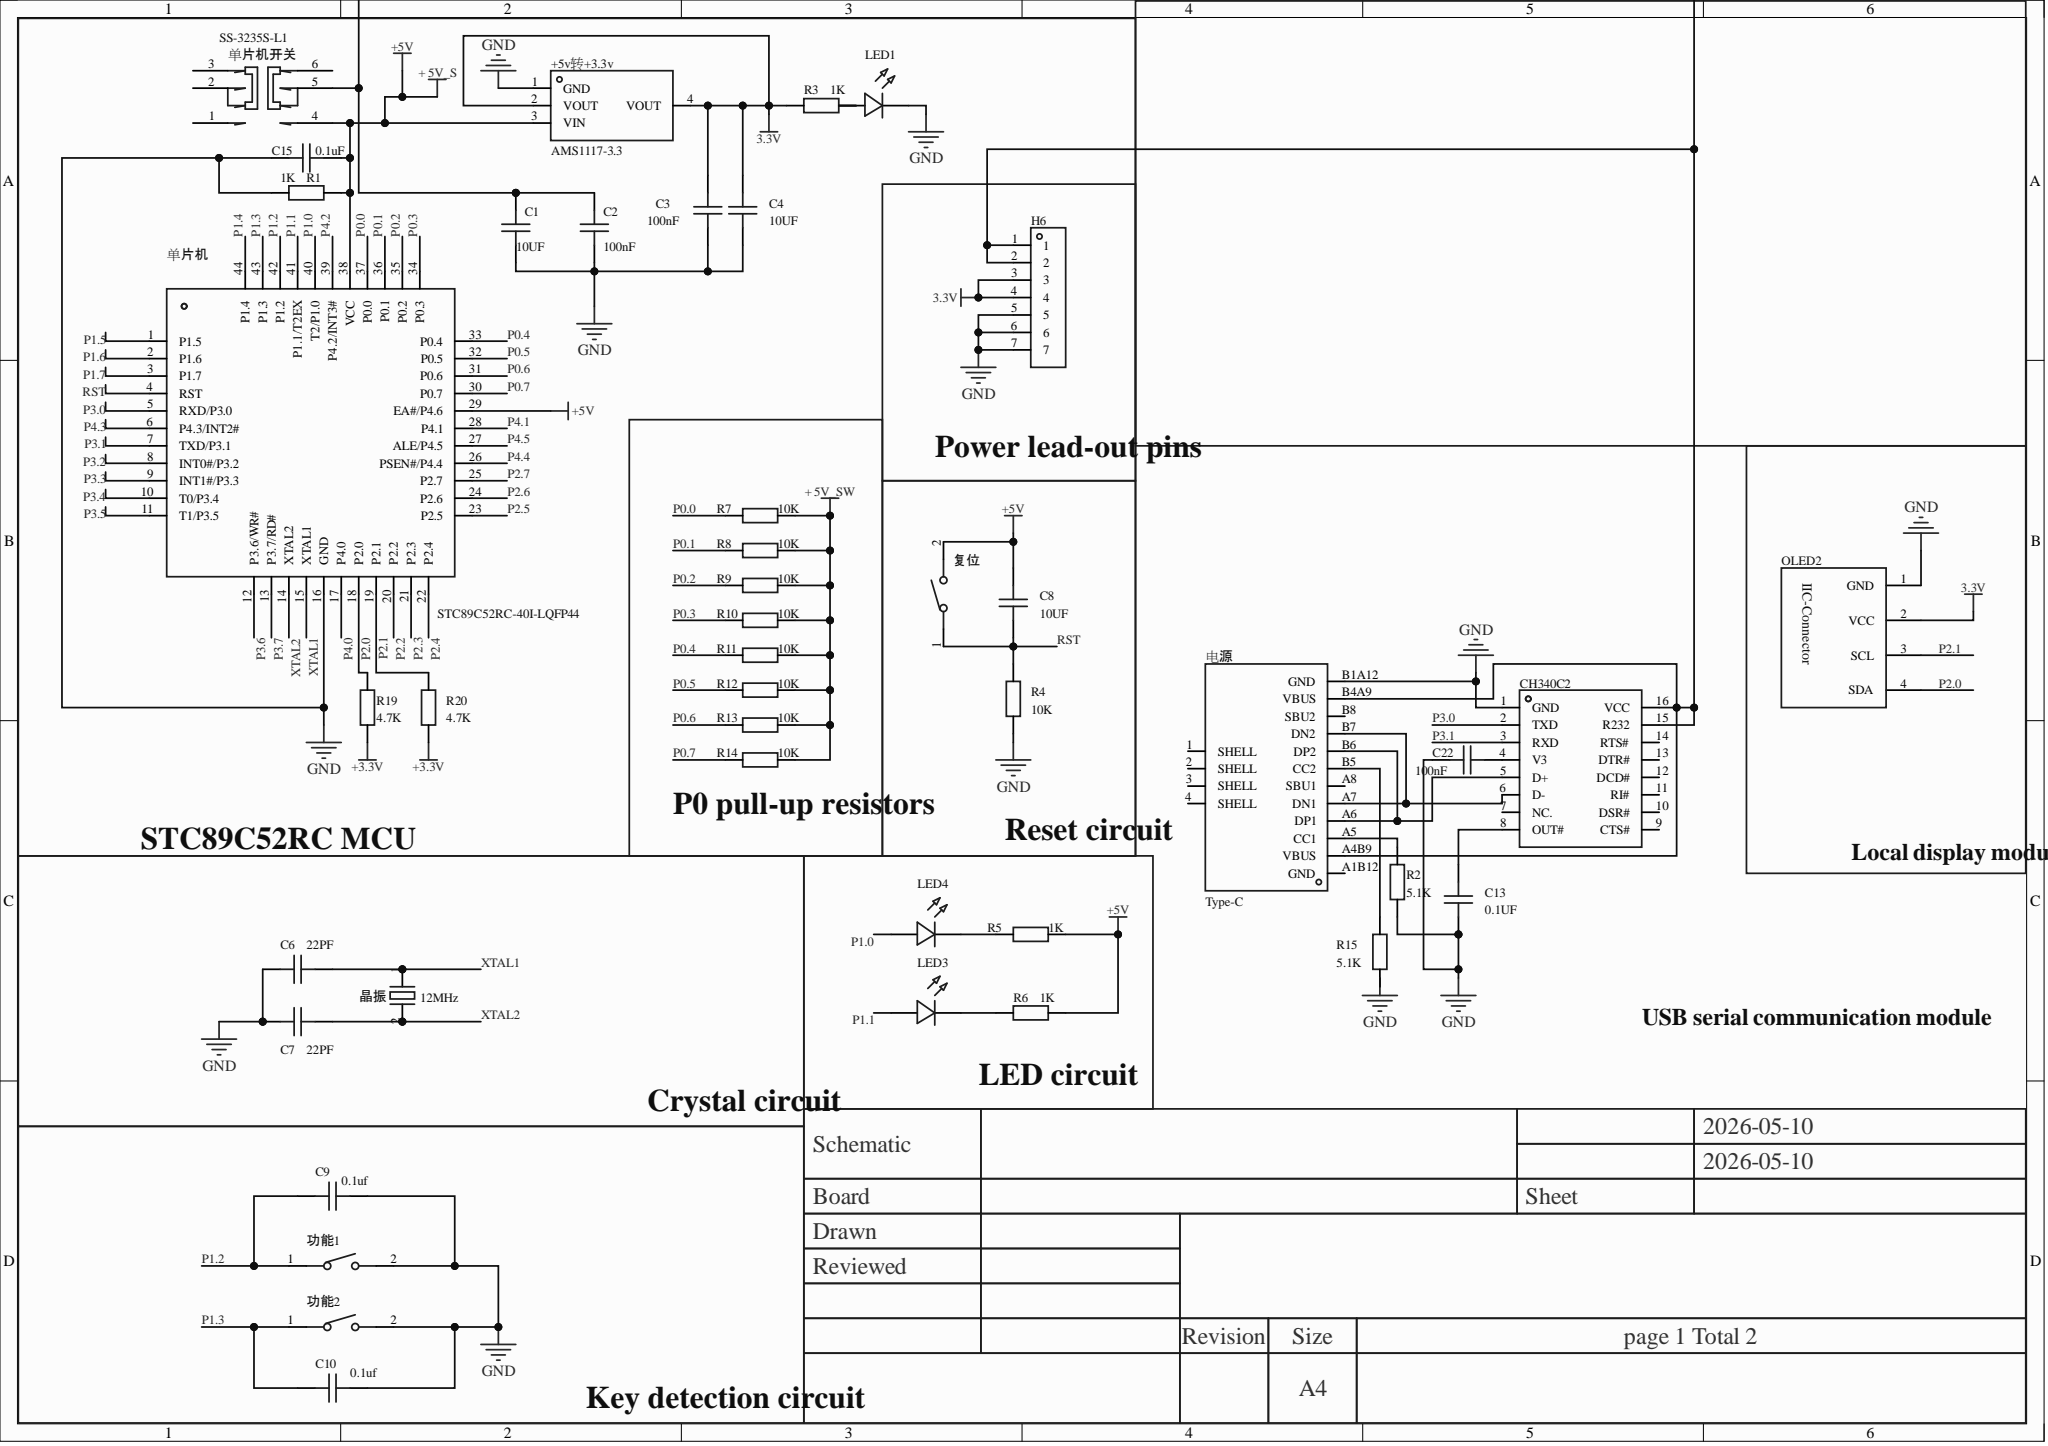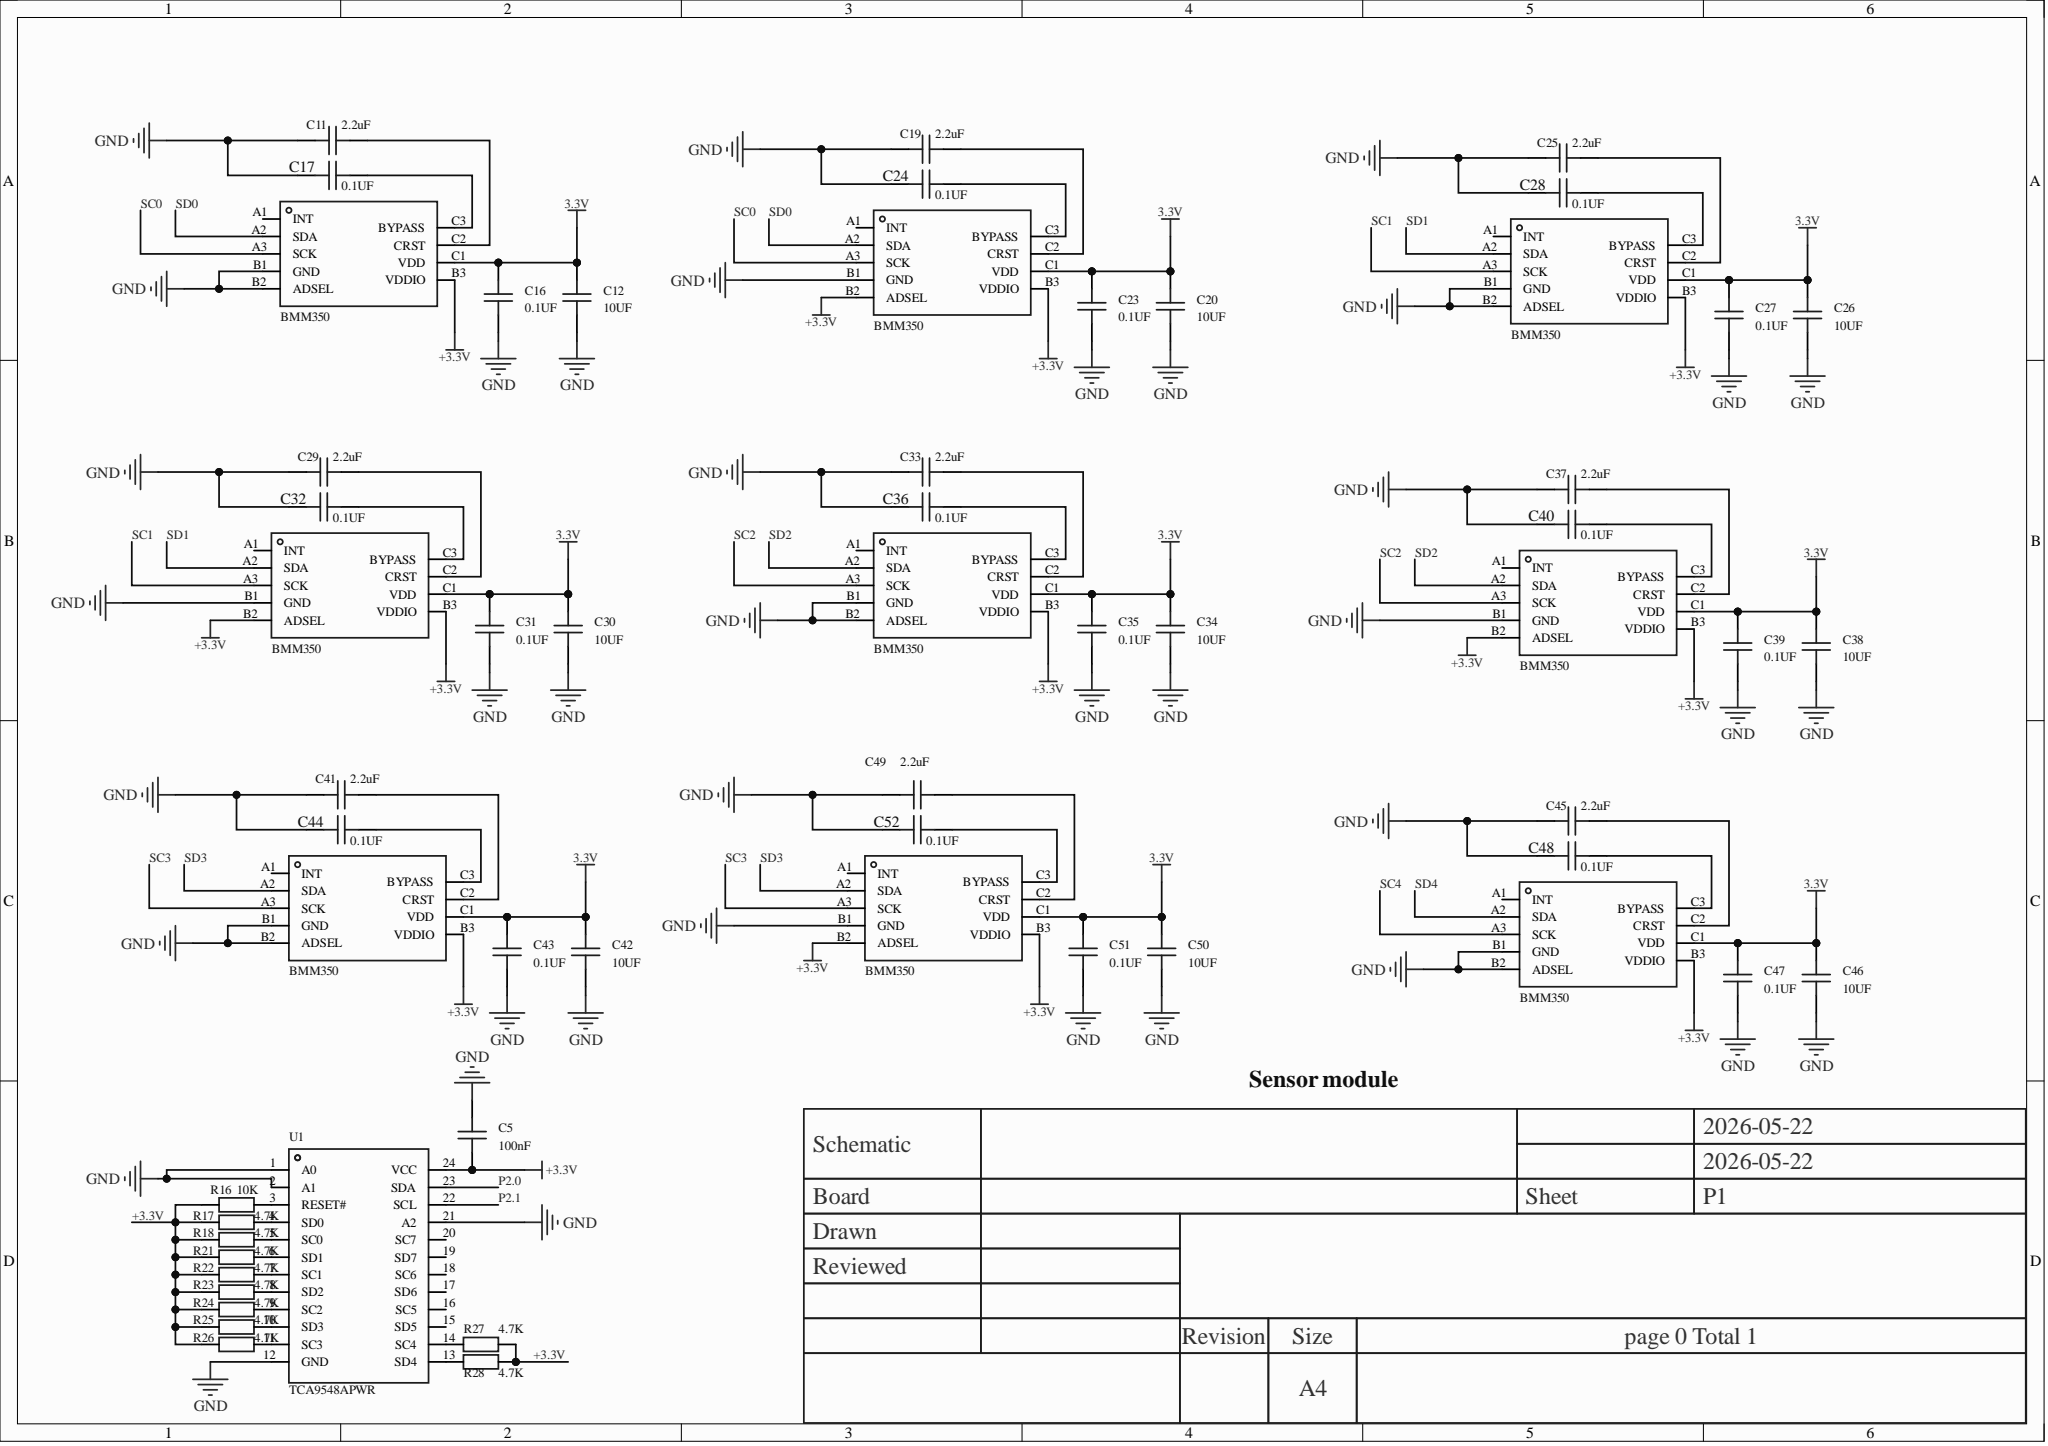Circuit board | Altium Designer | 101 parts | 69 nets
Bill of materials:
Comment,Description,Designator,Footprint,LibRef,Quantity
"AMS1117-3.3","Output type: fixed; working voltage: 15V; output voltage: 3.3V; output current: 1A; PSRR: 72dB@(120Hz); output polarity: positive;","+5v转+3.3v","SOT-223-3_L6.5-W3.4-P2.30-LS7.0-BR","AMS1117-3.3_C6186","1"
"10UF","","C1, C4, C8, C12, C20, C26, C30, C34, C38, C42, C46, C50","C0805","CAP_0805","12"
"100nF","","C2, C3, C5","C0805","CAP_0805","3"
"22PF","","C6, C7","C0805","CAP_0805","2"
"0.1uf","","C9, C10, C13, C15, C16, C17, C23, C24, C27, C28, C31, C32, C35, C36, C39, C40, C43, C44, C47, C48, C51, C52","C0805","CAP_0805","22"
"2.2uF","Capacitance: 2.2uF; tolerance: ±10%; rated voltage: 6.3V; dielectric (temperature coefficient): X7R;","C11, C19, C25, C29, C33, C37, C41, C45, C49","C0805","CGB4B3X7R0J225K055AB","9"
"100nF","","C22","C0603","CAP_0603","1"
"CH340C","Application function: transceiver; USB protocol version: USB 2.0; data rate: 2Mbps;","CH340C2","SOP-16_L10.0-W3.9-P1.27-LS6.0-BL","CH340C","1"
"","","H6","HDR-TH_7P-P2.54-V-M","HDR-M_2.54_1x7P","1"
"","","LED1, LED3, LED4","LED_0805","LED_0805-G","3"
"0.96OLED_4P_MODULE_JX","","OLED2","0.96OLED_4P","0.96OLED_4P_MODULE_JX","1"
"1K","","R1, R3, R5, R6","R0805","Res_0805","4"
"5.1K","","R2, R15","R0603","Res_0603","2"
"10K","","R4, R7, R8, R9, R10, R11, R12, R13, R14, R16","R0805","Res_0805","10"
"4.7K","","R17, R18, R21, R22, R23, R24, R25, R26, R27, R28","R0805","Res_0805","10"
"4.7K","","R19, R20","R0603","Res_0603","2"
"TCA9548APWR","TCA9548A 8-channel, 1.65V to 5.5V I2C/SMBus switch with reset and voltage translation","U1","TSSOP-24_L7.8-W4.4-P0.65-LS6.4-BL","TCA9548APWR","1"
"BMM350","","U2, U3, U4, U5, U6, U7, U8, U9, U10","WLCSP-9_L1.3-W1.3-R3-C3-P0.40-TL","BMM350","9"
"Tact switch 3*4*H","","功能1, 功能2, 复位","SW-SMD_L4.0-W2.9-LS5.0","轻触按键3*4*H","3"
"STC89C52RC-40I-LQFP44","CPU core: 51 family;","单片机","LQFP-44_L10.0-W10.0-P0.80-LS12.0-BL","STC89C52RC-40I-LQFP44","1"
"SS-3235S-L1","Circuit: DPDT; mounting: flat mount; switch colour: black; rated current: 50mA; rated voltage: 12V; service life: 1万 cycles;","单片机开关","SW-SMD_SS-3235S-LX","SS-3235S-L1","1"
"12MHz","Frequency: 12MHz; frequency tolerance at room temperature: ±30ppm; load capacitance: 18pF; frequency stability: ±35ppm;","晶振","CRYSTAL-SMD_L11.4-W4.7-LS12.7","ABLS-12.000MHZ-B4H-T","1"
"Type-C","","电源","USB-C-SMD_TYPE-C16PIN","Type-C-TOP_1","1"
Netlist (Protel format):
[
+5v转+3.3v
SOT-223-3_L6.5-W3.4-P2.30-LS7.0-BR
AMS1117-3.3



]
[
C1
C0805
10UF



]
[
C2
C0805
100nF



]
[
C3
C0805
100nF



]
[
C4
C0805
10UF



]
[
C5
C0805
100nF



]
[
C6
C0805
22PF



]
[
C7
C0805
22PF



]
[
C8
C0805
10UF



]
[
C9
C0805
0.1uf



]
[
C10
C0805
0.1uf



]
[
C11
C0805
2.2uF



]
[
C12
C0805
10UF



]
[
C13
C0805
0.1UF



]
[
C15
C0805
0.1uF



]
[
C16
C0805
0.1UF



]
[
C17
C0805
0.1UF



]
[
C19
C0805
2.2uF



]
[
C20
C0805
10UF



]
[
C22
C0603
100nF



]
[
C23
C0805
0.1UF



]
[
C24
C0805
0.1UF



]
[
C25
C0805
2.2uF



]
[
C26
C0805
10UF



]
[
C27
C0805
0.1UF



]
[
C28
C0805
0.1UF



]
[
C29
C0805
2.2uF



]
[
C30
C0805
10UF



]
[
C31
C0805
0.1UF



]
[
C32
C0805
0.1UF



]
[
C33
C0805
2.2uF



]
[
C34
C0805
10UF



]
[
C35
C0805
0.1UF



]
[
C36
C0805
0.1UF



]
[
C37
C0805
2.2uF



]
[
C38
C0805
10UF



]
[
C39
C0805
0.1UF



]
[
C40
C0805
0.1UF



]
[
C41
C0805
2.2uF



]
[
C42
C0805
10UF



]
[
C43
C0805
0.1UF



]
[
C44
C0805
0.1UF



]
[
C45
C0805
2.2uF



]
[
C46
C0805
10UF



]
[
C47
C0805
0.1UF



]
[
C48
C0805
0.1UF



]
[
C49
C0805
2.2uF



]
[
C50
C0805
10UF



]
[
C51
C0805
0.1UF



]
[
C52
C0805
0.1UF



]
[
CH340C2
SOP-16_L10.0-W3.9-P1.27-LS6.0-BL
CH340C



]
[
H6
HDR-TH_7P-P2.54-V-M




]
[
LED1
LED_0805




]
[
LED3
LED_0805




]
[
LED4
LED_0805




]
[
OLED2
0.96OLED_4P
0.96OLED_4P_MODULE_JX



]
[
R1
R0805
1K



]
[
R2
R0603
5.1K



]
[
R3
R0805
1K



]
[
R4
R0805
10K



]
[
R5
R0805
1K



]
[
R6
R0805
1K



]
[
R7
R0805
10K



]
[
R8
R0805
10K



]
[
R9
R0805
10K



]
[
R10
R0805
10K



]
[
R11
R0805
10K



]
[
R12
R0805
10K



]
[
R13
R0805
10K



]
[
R14
R0805
10K



]
[
R15
R0603
5.1K



]
[
R16
R0805
10K



]
[
R17
R0805
4.7K



]
[
R18
R0805
4.7K



]
[
R19
R0603
4.7K



]
[
R20
R0603
4.7K



]
[
R21
R0805
4.7K



]
[
R22
R0805
4.7K



]
[
R23
R0805
4.7K



]
[
R24
R0805
4.7K



]
[
R25
R0805
4.7K



]
[
R26
R0805
4.7K



]
[
R27
R0805
4.7K



]
[
R28
R0805
4.7K



]
[
U1
TSSOP-24_L7.8-W4.4-P0.65-LS6.4-BL
TCA9548APWR



]
[
U2
WLCSP-9_L1.3-W1.3-R3-C3-P0.40-TL
BMM350



]
[
U3
WLCSP-9_L1.3-W1.3-R3-C3-P0.40-TL
BMM350



]
[
U4
WLCSP-9_L1.3-W1.3-R3-C3-P0.40-TL
BMM350



]
[
U5
WLCSP-9_L1.3-W1.3-R3-C3-P0.40-TL
BMM350



]
[
U6
WLCSP-9_L1.3-W1.3-R3-C3-P0.40-TL
BMM350



]
[
U7
WLCSP-9_L1.3-W1.3-R3-C3-P0.40-TL
BMM350



]
[
U8
WLCSP-9_L1.3-W1.3-R3-C3-P0.40-TL
BMM350



]
[
U9
WLCSP-9_L1.3-W1.3-R3-C3-P0.40-TL
BMM350



]
[
U10
WLCSP-9_L1.3-W1.3-R3-C3-P0.40-TL
BMM350



]
[
功能1
SW-SMD_L4.0-W2.9-LS5.0
Tact switch 3*4*H



]
[
功能2
SW-SMD_L4.0-W2.9-LS5.0
Tact switch 3*4*H



]
[
单片机
LQFP-44_L10.0-W10.0-P0.80-LS12.0-BL
STC89C52RC-40I-LQFP44



]
[
单片机开关
SW-SMD_SS-3235S-LX
SS-3235S-L1



]
[
复位
SW-SMD_L4.0-W2.9-LS5.0
Tact switch 3*4*H



]
[
晶振
CRYSTAL-SMD_L11.4-W4.7-LS12.7
12MHz



]
[
电源
USB-C-SMD_TYPE-C16PIN
Type-C



]
(
XTAL2
C7-1
单片机-14
晶振-2
)
(
XTAL1
C6-1
单片机-15
晶振-1
)
(
SD3
U8-A2
U10-A2
)
(
SD2
U6-A2
U7-A2
)
(
SD1
U4-A2
U5-A2
)
(
SD0
U2-A2
U3-A2
)
(
SC3
U8-A3
U10-A3
)
(
SC2
U6-A3
U7-A3
)
(
SC1
U4-A3
U5-A3
)
(
SC0
U2-A3
U3-A3
)
(
RST
C8-2
R4-2
单片机-4
复位-1
)
(
P3.1
CH340C2-3
单片机-7
)
(
P3.0
CH340C2-2
单片机-5
)
(
P2.1
OLED2-3
R20-2
U1-22
单片机-19
)
(
P2.0
OLED2-4
R19-2
U1-23
单片机-18
)
(
P1.3
C10-2
功能2-1
单片机-43
)
(
P1.2
C9-2
功能1-1
单片机-42
)
(
P1.1
LED3-2
单片机-41
)
(
P1.0
LED4-2
单片机-40
)
(
P0.7
R14-1
单片机-30
)
(
P0.6
R13-1
单片机-31
)
(
P0.5
R12-1
单片机-32
)
(
P0.4
R11-1
单片机-33
)
(
P0.3
R10-1
单片机-34
)
(
P0.2
R9-1
单片机-35
)
(
P0.1
R8-1
单片机-36
)
(
P0.0
R7-1
单片机-37
)
(
NetR28_1
R28-1
U1-13
)
(
NetR27_1
R27-1
U1-14
)
(
NetR26_2
R26-2
U1-11
)
(
NetR25_2
R25-2
U1-10
)
(
NetR24_2
R24-2
U1-9
)
(
NetR23_2
R23-2
U1-8
)
(
NetR22_2
R22-2
U1-7
)
(
NetR21_2
R21-2
U1-6
)
(
NetR18_2
R18-2
U1-5
)
(
NetR17_2
R17-2
U1-4
)
(
NetR16_2
R16-2
U1-3
)
(
NetR15_2
R15-2
电源-B5
)
(
NetR2_2
R2-2
电源-A5
)
(
NetLED4_1
LED4-1
R5-1
)
(
NetLED3_1
LED3-1
R6-1
)
(
NetLED1_2
LED1-2
R3-2
)
(
NetCH340C2_6
CH340C2-6
电源-A7
电源-B7
)
(
NetCH340C2_5
CH340C2-5
电源-A6
电源-B6
)
(
NetC52_2
C52-2
U10-C3
)
(
NetC49_1
C49-1
U10-C2
)
(
NetC48_2
C48-2
U9-C3
)
(
NetC45_1
C45-1
U9-C2
)
(
NetC44_2
C44-2
U8-C3
)
(
NetC41_1
C41-1
U8-C2
)
(
NetC40_2
C40-2
U7-C3
)
(
NetC37_1
C37-1
U7-C2
)
(
NetC36_2
C36-2
U6-C3
)
(
NetC33_1
C33-1
U6-C2
)
(
NetC32_2
C32-2
U5-C3
)
(
NetC29_1
C29-1
U5-C2
)
(
NetC28_2
C28-2
U4-C3
)
(
NetC25_1
C25-1
U4-C2
)
(
NetC24_2
C24-2
U3-C3
)
(
NetC22_2
C22-2
CH340C2-4
)
(
NetC19_1
C19-1
U3-C2
)
(
NetC17_2
C17-2
U2-C3
)
(
NetC13_2
C13-2
CH340C2-8
)
(
NetC11_1
C11-1
U2-C2
)
(
NetC1_2
C1-2
C2-2
CH340C2-15
CH340C2-16
H6-1
H6-2
单片机开关-5
电源-A4B9
电源-B4A9
)
(
GND
+5v转+3.3v-1
C1-1
C2-1
C3-1
C4-1
C5-2
C6-2
C7-2
C9-1
C10-1
C11-2
C12-2
C13-1
C15-1
C16-1
C17-1
C19-2
C20-2
C22-1
C23-1
C24-1
C25-2
C26-2
C27-1
C28-1
C29-2
C30-2
C31-1
C32-1
C33-2
C34-2
C35-1
C36-1
C37-2
C38-2
C39-1
C40-1
C41-2
C42-2
C43-1
C44-1
C45-2
C46-2
C47-1
C48-1
C49-2
C50-2
C51-1
C52-1
CH340C2-1
H6-5
H6-6
H6-7
LED1-1
OLED2-1
R1-1
R2-1
R4-1
R15-1
U1-1
U1-2
U1-12
U1-21
U2-B1
U2-B2
U3-B1
U4-B1
U4-B2
U5-B1
U6-B1
U6-B2
U7-B1
U8-B1
U8-B2
U9-B1
U9-B2
U10-B1
功能1-2
功能2-2
单片机-16
电源-B1A12
)
(
+3.3V
+5v转+3.3v-3
C5-1
C8-1
C15-2
R1-2
R5-2
R6-2
R7-2
R8-2
R9-2
R10-2
R11-2
R12-2
R13-2
R14-2
R16-1
R17-1
R18-1
R19-1
R20-1
R21-1
R22-1
R23-1
R24-1
R25-1
R26-1
R27-2
R28-2
U1-24
U2-B3
U3-B2
U3-B3
U4-B3
U5-B2
U5-B3
U6-B3
U7-B2
U7-B3
U8-B3
U9-B3
U10-B2
U10-B3
单片机-29
单片机-38
单片机开关-4
复位-2
)
(
3.3V
+5v转+3.3v-2
+5v转+3.3v-4
C3-2
C4-2
C12-1
C16-2
C20-1
C23-2
C26-1
C27-2
C30-1
C31-2
C34-1
C35-2
C38-1
C39-2
C42-1
C43-2
C46-1
C47-2
C50-1
C51-2
H6-3
H6-4
OLED2-2
R3-1
U2-C1
U3-C1
U4-C1
U5-C1
U6-C1
U7-C1
U8-C1
U9-C1
U10-C1
)